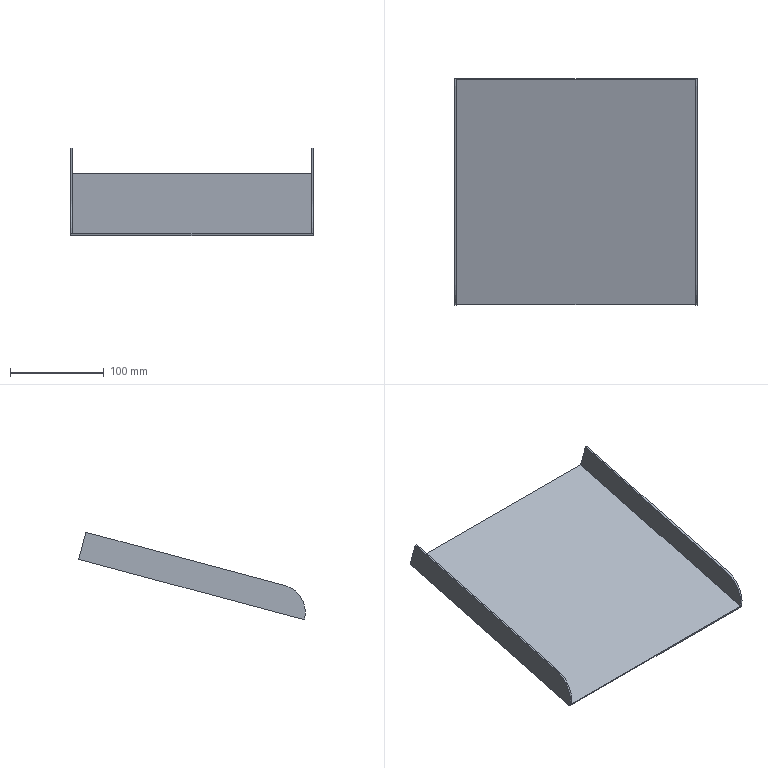Part | NX | features solid 2 | 1 solid | 12 faces | box 259.608 x 242.504 x 93.683 mm | volume 157032 mm3 | plane 10 | cylinder 2 | commonest cylinder face diameters 60 x2
STEP:
#1=CARTESIAN_POINT('',(828.,-707.325,-528.971));
#2=VERTEX_POINT('',#1);
#3=CARTESIAN_POINT('',(828.,-948.742,-593.658));
#4=VERTEX_POINT('',#3);
#5=CARTESIAN_POINT('',(828.,-784.599,-549.676));
#6=DIRECTION('',(0.,-0.9659,-0.2588));
#7=VECTOR('',#6,1000.);
#8=LINE('',#5,#7);
#9=EDGE_CURVE('',#2,#4,#8,.T.);
#10=ORIENTED_EDGE('',*,*,#9,.F.);
#11=CARTESIAN_POINT('',(572.392,-707.325,-528.971));
#12=VERTEX_POINT('',#11);
#13=CARTESIAN_POINT('',(818.,-707.325,-528.971));
#14=DIRECTION('',(1.,0.,0.));
#15=VECTOR('',#14,1000.);
#16=LINE('',#13,#15);
#17=EDGE_CURVE('',#2,#12,#16,.F.);
#18=ORIENTED_EDGE('',*,*,#17,.T.);
#19=CARTESIAN_POINT('',(572.392,-948.742,-593.658));
#20=VERTEX_POINT('',#19);
#21=CARTESIAN_POINT('',(572.392,-766.757,-544.895));
#22=DIRECTION('',(0.,0.9659,0.2588));
#23=VECTOR('',#22,1000.);
#24=LINE('',#21,#23);
#25=EDGE_CURVE('',#12,#20,#24,.F.);
#26=ORIENTED_EDGE('',*,*,#25,.T.);
#27=CARTESIAN_POINT('',(570.392,-948.742,-593.658));
#28=VERTEX_POINT('',#27);
#29=CARTESIAN_POINT('',(594.206,-948.742,-593.658));
#30=DIRECTION('',(-1.,0.,0.));
#31=VECTOR('',#30,1000.);
#32=LINE('',#29,#31);
#33=EDGE_CURVE('',#28,#20,#32,.F.);
#34=ORIENTED_EDGE('',*,*,#33,.F.);
#35=CARTESIAN_POINT('',(570.392,-948.807,-593.675));
#36=VERTEX_POINT('',#35);
#37=CARTESIAN_POINT('',(570.392,-795.624,-552.63));
#38=DIRECTION('',(0.,0.9659,0.2588));
#39=VECTOR('',#38,1000.);
#40=LINE('',#37,#39);
#41=EDGE_CURVE('',#28,#36,#40,.F.);
#42=ORIENTED_EDGE('',*,*,#41,.T.);
#43=CARTESIAN_POINT('',(830.,-948.807,-593.675));
#44=VERTEX_POINT('',#43);
#45=CARTESIAN_POINT('',(818.,-948.807,-593.675));
#46=DIRECTION('',(1.,0.,0.));
#47=VECTOR('',#46,1000.);
#48=LINE('',#45,#47);
#49=EDGE_CURVE('',#44,#36,#48,.F.);
#50=ORIENTED_EDGE('',*,*,#49,.F.);
#51=CARTESIAN_POINT('',(830.,-948.742,-593.658));
#52=VERTEX_POINT('',#51);
#53=CARTESIAN_POINT('',(830.,-784.599,-549.676));
#54=DIRECTION('',(0.,-0.9659,-0.2588));
#55=VECTOR('',#54,1000.);
#56=LINE('',#53,#55);
#57=EDGE_CURVE('',#52,#44,#56,.T.);
#58=ORIENTED_EDGE('',*,*,#57,.F.);
#59=CARTESIAN_POINT('',(830.,-948.742,-593.658));
#60=DIRECTION('',(1.,0.,0.));
#61=VECTOR('',#60,1000.);
#62=LINE('',#59,#61);
#63=EDGE_CURVE('',#4,#52,#62,.T.);
#64=ORIENTED_EDGE('',*,*,#63,.F.);
#65=EDGE_LOOP('',(#10,#18,#26,#34,#42,#50,#58,#64));
#66=FACE_BOUND('',#65,.T.);
#67=CARTESIAN_POINT('',(818.,-784.599,-549.676));
#68=DIRECTION('',(0.,-0.2588,0.9659));
#69=DIRECTION('',(1.,0.,0.));
#70=AXIS2_PLACEMENT_3D('',#67,#68,#69);
#71=PLANE('',#70);
#72=ADVANCED_FACE('',(#66),#71,.T.);
#73=ORIENTED_EDGE('',*,*,#17,.F.);
#74=CARTESIAN_POINT('',(828.,-714.572,-501.925));
#75=VERTEX_POINT('',#74);
#76=CARTESIAN_POINT('',(828.,-706.808,-530.902));
#77=DIRECTION('',(0.,0.2588,-0.9659));
#78=VECTOR('',#77,1000.);
#79=LINE('',#76,#78);
#80=EDGE_CURVE('',#2,#75,#79,.F.);
#81=ORIENTED_EDGE('',*,*,#80,.T.);
#82=CARTESIAN_POINT('',(830.,-714.572,-501.925));
#83=VERTEX_POINT('',#82);
#84=CARTESIAN_POINT('',(818.,-714.572,-501.925));
#85=DIRECTION('',(-1.,0.,0.));
#86=VECTOR('',#85,1000.);
#87=LINE('',#84,#86);
#88=EDGE_CURVE('',#83,#75,#87,.T.);
#89=ORIENTED_EDGE('',*,*,#88,.F.);
#90=CARTESIAN_POINT('',(830.,-706.808,-530.902));
#91=VERTEX_POINT('',#90);
#92=CARTESIAN_POINT('',(830.,-706.808,-530.902));
#93=DIRECTION('',(0.,0.2588,-0.9659));
#94=VECTOR('',#93,1000.);
#95=LINE('',#92,#94);
#96=EDGE_CURVE('',#91,#83,#95,.F.);
#97=ORIENTED_EDGE('',*,*,#96,.F.);
#98=CARTESIAN_POINT('',(570.392,-706.808,-530.902));
#99=VERTEX_POINT('',#98);
#100=CARTESIAN_POINT('',(818.,-706.808,-530.902));
#101=DIRECTION('',(1.,0.,0.));
#102=VECTOR('',#101,1000.);
#103=LINE('',#100,#102);
#104=EDGE_CURVE('',#91,#99,#103,.F.);
#105=ORIENTED_EDGE('',*,*,#104,.T.);
#106=CARTESIAN_POINT('',(570.392,-714.572,-501.925));
#107=VERTEX_POINT('',#106);
#108=CARTESIAN_POINT('',(570.392,-706.808,-530.902));
#109=DIRECTION('',(0.,-0.2588,0.9659));
#110=VECTOR('',#109,1000.);
#111=LINE('',#108,#110);
#112=EDGE_CURVE('',#99,#107,#111,.T.);
#113=ORIENTED_EDGE('',*,*,#112,.T.);
#114=CARTESIAN_POINT('',(572.392,-714.572,-501.925));
#115=VERTEX_POINT('',#114);
#116=CARTESIAN_POINT('',(818.,-714.572,-501.925));
#117=DIRECTION('',(-1.,0.,0.));
#118=VECTOR('',#117,1000.);
#119=LINE('',#116,#118);
#120=EDGE_CURVE('',#107,#115,#119,.F.);
#121=ORIENTED_EDGE('',*,*,#120,.T.);
#122=CARTESIAN_POINT('',(572.392,-706.808,-530.902));
#123=DIRECTION('',(0.,-0.2588,0.9659));
#124=VECTOR('',#123,1000.);
#125=LINE('',#122,#124);
#126=EDGE_CURVE('',#12,#115,#125,.T.);
#127=ORIENTED_EDGE('',*,*,#126,.F.);
#128=EDGE_LOOP('',(#73,#81,#89,#97,#105,#113,#121,#127));
#129=FACE_BOUND('',#128,.T.);
#130=CARTESIAN_POINT('',(818.,-706.808,-530.902));
#131=DIRECTION('',(0.,0.9659,0.2588));
#132=DIRECTION('',(-1.,0.,0.));
#133=AXIS2_PLACEMENT_3D('',#130,#131,#132);
#134=PLANE('',#133);
#135=ADVANCED_FACE('',(#129),#134,.T.);
#136=CARTESIAN_POINT('',(830.,-948.289,-595.607));
#137=VERTEX_POINT('',#136);
#138=CARTESIAN_POINT('',(830.,-948.289,-595.607));
#139=DIRECTION('',(0.,-0.2588,0.9659));
#140=VECTOR('',#139,1000.);
#141=LINE('',#138,#140);
#142=EDGE_CURVE('',#137,#44,#141,.T.);
#143=ORIENTED_EDGE('',*,*,#142,.F.);
#144=CARTESIAN_POINT('',(830.,-784.082,-551.608));
#145=DIRECTION('',(0.,-0.9659,-0.2588));
#146=VECTOR('',#145,1000.);
#147=LINE('',#144,#146);
#148=EDGE_CURVE('',#91,#137,#147,.T.);
#149=ORIENTED_EDGE('',*,*,#148,.F.);
#150=ORIENTED_EDGE('',*,*,#96,.T.);
#151=CARTESIAN_POINT('',(830.,-927.076,-558.865));
#152=VERTEX_POINT('',#151);
#153=CARTESIAN_POINT('',(830.,-791.846,-522.63));
#154=DIRECTION('',(0.,-0.9659,-0.2588));
#155=VECTOR('',#154,1000.);
#156=LINE('',#153,#155);
#157=EDGE_CURVE('',#83,#152,#156,.T.);
#158=ORIENTED_EDGE('',*,*,#157,.T.);
#159=CARTESIAN_POINT('',(830.,-919.311,-587.843));
#160=DIRECTION('',(-1.,0.,0.));
#161=DIRECTION('',(0.,-0.2588,0.9659));
#162=AXIS2_PLACEMENT_3D('',#159,#160,#161);
#163=CIRCLE('',#162,30.);
#164=EDGE_CURVE('',#152,#52,#163,.F.);
#165=ORIENTED_EDGE('',*,*,#164,.T.);
#166=ORIENTED_EDGE('',*,*,#57,.T.);
#167=EDGE_LOOP('',(#143,#149,#150,#158,#165,#166));
#168=FACE_BOUND('',#167,.T.);
#169=CARTESIAN_POINT('',(830.,-784.082,-551.608));
#170=DIRECTION('',(-1.,0.,0.));
#171=DIRECTION('',(0.,-0.9659,-0.2588));
#172=AXIS2_PLACEMENT_3D('',#169,#170,#171);
#173=PLANE('',#172);
#174=ADVANCED_FACE('',(#168),#173,.F.);
#175=ORIENTED_EDGE('',*,*,#142,.T.);
#176=ORIENTED_EDGE('',*,*,#49,.T.);
#177=CARTESIAN_POINT('',(570.392,-948.289,-595.607));
#178=VERTEX_POINT('',#177);
#179=CARTESIAN_POINT('',(570.392,-936.311,-640.312));
#180=DIRECTION('',(0.,0.2588,-0.9659));
#181=VECTOR('',#180,1000.);
#182=LINE('',#179,#181);
#183=EDGE_CURVE('',#178,#36,#182,.F.);
#184=ORIENTED_EDGE('',*,*,#183,.F.);
#185=CARTESIAN_POINT('',(818.,-948.289,-595.607));
#186=DIRECTION('',(-1.,0.,0.));
#187=VECTOR('',#186,1000.);
#188=LINE('',#185,#187);
#189=EDGE_CURVE('',#137,#178,#188,.T.);
#190=ORIENTED_EDGE('',*,*,#189,.F.);
#191=EDGE_LOOP('',(#175,#176,#184,#190));
#192=FACE_BOUND('',#191,.T.);
#193=CARTESIAN_POINT('',(818.,-948.289,-595.607));
#194=DIRECTION('',(0.,0.9659,0.2588));
#195=DIRECTION('',(-1.,0.,0.));
#196=AXIS2_PLACEMENT_3D('',#193,#194,#195);
#197=PLANE('',#196);
#198=ADVANCED_FACE('',(#192),#197,.F.);
#199=ORIENTED_EDGE('',*,*,#41,.F.);
#200=CARTESIAN_POINT('',(570.392,-927.076,-558.865));
#201=VERTEX_POINT('',#200);
#202=CARTESIAN_POINT('',(570.392,-919.311,-587.843));
#203=DIRECTION('',(-1.,0.,0.));
#204=DIRECTION('',(0.,0.,1.));
#205=AXIS2_PLACEMENT_3D('',#202,#203,#204);
#206=CIRCLE('',#205,30.);
#207=EDGE_CURVE('',#28,#201,#206,.T.);
#208=ORIENTED_EDGE('',*,*,#207,.T.);
#209=CARTESIAN_POINT('',(570.392,-791.846,-522.63));
#210=DIRECTION('',(0.,0.9659,0.2588));
#211=VECTOR('',#210,1000.);
#212=LINE('',#209,#211);
#213=EDGE_CURVE('',#107,#201,#212,.F.);
#214=ORIENTED_EDGE('',*,*,#213,.F.);
#215=ORIENTED_EDGE('',*,*,#112,.F.);
#216=CARTESIAN_POINT('',(570.392,-795.107,-554.562));
#217=DIRECTION('',(0.,0.9659,0.2588));
#218=VECTOR('',#217,1000.);
#219=LINE('',#216,#218);
#220=EDGE_CURVE('',#99,#178,#219,.F.);
#221=ORIENTED_EDGE('',*,*,#220,.T.);
#222=ORIENTED_EDGE('',*,*,#183,.T.);
#223=EDGE_LOOP('',(#199,#208,#214,#215,#221,#222));
#224=FACE_BOUND('',#223,.T.);
#225=CARTESIAN_POINT('',(570.392,-783.128,-599.267));
#226=DIRECTION('',(-1.,0.,0.));
#227=DIRECTION('',(0.,-0.9397,-0.342));
#228=AXIS2_PLACEMENT_3D('',#225,#226,#227);
#229=PLANE('',#228);
#230=ADVANCED_FACE('',(#224),#229,.T.);
#231=ORIENTED_EDGE('',*,*,#220,.F.);
#232=ORIENTED_EDGE('',*,*,#104,.F.);
#233=ORIENTED_EDGE('',*,*,#148,.T.);
#234=ORIENTED_EDGE('',*,*,#189,.T.);
#235=EDGE_LOOP('',(#231,#232,#233,#234));
#236=FACE_BOUND('',#235,.T.);
#237=CARTESIAN_POINT('',(818.,-784.082,-551.608));
#238=DIRECTION('',(0.,-0.2588,0.9659));
#239=DIRECTION('',(1.,0.,0.));
#240=AXIS2_PLACEMENT_3D('',#237,#238,#239);
#241=PLANE('',#240);
#242=ADVANCED_FACE('',(#236),#241,.F.);
#243=ORIENTED_EDGE('',*,*,#213,.T.);
#244=CARTESIAN_POINT('',(572.392,-927.076,-558.865));
#245=VERTEX_POINT('',#244);
#246=CARTESIAN_POINT('',(594.206,-927.076,-558.865));
#247=DIRECTION('',(-1.,0.,0.));
#248=VECTOR('',#247,1000.);
#249=LINE('',#246,#248);
#250=EDGE_CURVE('',#201,#245,#249,.F.);
#251=ORIENTED_EDGE('',*,*,#250,.T.);
#252=CARTESIAN_POINT('',(572.392,-791.846,-522.63));
#253=DIRECTION('',(0.,0.9659,0.2588));
#254=VECTOR('',#253,1000.);
#255=LINE('',#252,#254);
#256=EDGE_CURVE('',#115,#245,#255,.F.);
#257=ORIENTED_EDGE('',*,*,#256,.F.);
#258=ORIENTED_EDGE('',*,*,#120,.F.);
#259=EDGE_LOOP('',(#243,#251,#257,#258));
#260=FACE_BOUND('',#259,.T.);
#261=CARTESIAN_POINT('',(594.206,-791.846,-522.63));
#262=DIRECTION('',(0.,0.2588,-0.9659));
#263=DIRECTION('',(0.,-0.9659,-0.2588));
#264=AXIS2_PLACEMENT_3D('',#261,#262,#263);
#265=PLANE('',#264);
#266=ADVANCED_FACE('',(#260),#265,.F.);
#267=ORIENTED_EDGE('',*,*,#25,.F.);
#268=ORIENTED_EDGE('',*,*,#126,.T.);
#269=ORIENTED_EDGE('',*,*,#256,.T.);
#270=CARTESIAN_POINT('',(572.392,-919.311,-587.843));
#271=DIRECTION('',(-1.,0.,0.));
#272=DIRECTION('',(0.,0.,1.));
#273=AXIS2_PLACEMENT_3D('',#270,#271,#272);
#274=CIRCLE('',#273,30.);
#275=EDGE_CURVE('',#245,#20,#274,.F.);
#276=ORIENTED_EDGE('',*,*,#275,.T.);
#277=EDGE_LOOP('',(#267,#268,#269,#276));
#278=FACE_BOUND('',#277,.T.);
#279=CARTESIAN_POINT('',(572.392,-754.937,-589.006));
#280=DIRECTION('',(-1.,0.,0.));
#281=DIRECTION('',(0.,0.,1.));
#282=AXIS2_PLACEMENT_3D('',#279,#280,#281);
#283=PLANE('',#282);
#284=ADVANCED_FACE('',(#278),#283,.F.);
#285=ORIENTED_EDGE('',*,*,#207,.F.);
#286=ORIENTED_EDGE('',*,*,#33,.T.);
#287=ORIENTED_EDGE('',*,*,#275,.F.);
#288=ORIENTED_EDGE('',*,*,#250,.F.);
#289=EDGE_LOOP('',(#285,#286,#287,#288));
#290=FACE_BOUND('',#289,.T.);
#291=CARTESIAN_POINT('',(594.206,-919.311,-587.843));
#292=DIRECTION('',(-1.,0.,0.));
#293=DIRECTION('',(0.,-0.2588,0.9659));
#294=AXIS2_PLACEMENT_3D('',#291,#292,#293);
#295=CYLINDRICAL_SURFACE('',#294,30.);
#296=ADVANCED_FACE('',(#290),#295,.T.);
#297=CARTESIAN_POINT('',(828.,-927.076,-558.865));
#298=VERTEX_POINT('',#297);
#299=CARTESIAN_POINT('',(828.,-791.846,-522.63));
#300=DIRECTION('',(0.,0.9659,0.2588));
#301=VECTOR('',#300,1000.);
#302=LINE('',#299,#301);
#303=EDGE_CURVE('',#75,#298,#302,.F.);
#304=ORIENTED_EDGE('',*,*,#303,.T.);
#305=CARTESIAN_POINT('',(830.,-927.076,-558.865));
#306=DIRECTION('',(-1.,0.,0.));
#307=VECTOR('',#306,1000.);
#308=LINE('',#305,#307);
#309=EDGE_CURVE('',#298,#152,#308,.F.);
#310=ORIENTED_EDGE('',*,*,#309,.T.);
#311=ORIENTED_EDGE('',*,*,#157,.F.);
#312=ORIENTED_EDGE('',*,*,#88,.T.);
#313=EDGE_LOOP('',(#304,#310,#311,#312));
#314=FACE_BOUND('',#313,.T.);
#315=CARTESIAN_POINT('',(830.,-791.846,-522.63));
#316=DIRECTION('',(0.,0.2588,-0.9659));
#317=DIRECTION('',(0.,-0.9659,-0.2588));
#318=AXIS2_PLACEMENT_3D('',#315,#316,#317);
#319=PLANE('',#318);
#320=ADVANCED_FACE('',(#314),#319,.F.);
#321=ORIENTED_EDGE('',*,*,#80,.F.);
#322=ORIENTED_EDGE('',*,*,#9,.T.);
#323=CARTESIAN_POINT('',(828.,-919.311,-587.843));
#324=DIRECTION('',(-1.,0.,0.));
#325=DIRECTION('',(0.,-0.2588,0.9659));
#326=AXIS2_PLACEMENT_3D('',#323,#324,#325);
#327=CIRCLE('',#326,30.);
#328=EDGE_CURVE('',#4,#298,#327,.T.);
#329=ORIENTED_EDGE('',*,*,#328,.T.);
#330=ORIENTED_EDGE('',*,*,#303,.F.);
#331=EDGE_LOOP('',(#321,#322,#329,#330));
#332=FACE_BOUND('',#331,.T.);
#333=CARTESIAN_POINT('',(828.,-784.082,-551.608));
#334=DIRECTION('',(-1.,0.,0.));
#335=DIRECTION('',(0.,-0.2588,0.9659));
#336=AXIS2_PLACEMENT_3D('',#333,#334,#335);
#337=PLANE('',#336);
#338=ADVANCED_FACE('',(#332),#337,.T.);
#339=ORIENTED_EDGE('',*,*,#328,.F.);
#340=ORIENTED_EDGE('',*,*,#63,.T.);
#341=ORIENTED_EDGE('',*,*,#164,.F.);
#342=ORIENTED_EDGE('',*,*,#309,.F.);
#343=EDGE_LOOP('',(#339,#340,#341,#342));
#344=FACE_BOUND('',#343,.T.);
#345=CARTESIAN_POINT('',(830.,-919.311,-587.843));
#346=DIRECTION('',(1.,0.,0.));
#347=DIRECTION('',(0.,0.2588,-0.9659));
#348=AXIS2_PLACEMENT_3D('',#345,#346,#347);
#349=CYLINDRICAL_SURFACE('',#348,30.);
#350=ADVANCED_FACE('',(#344),#349,.T.);
#351=CLOSED_SHELL('',(#72,#135,#174,#198,#230,#242,#266,#284,#296,#320,#338,#350));
#352=MANIFOLD_SOLID_BREP('',#351);
#353=(LENGTH_UNIT()NAMED_UNIT(*)SI_UNIT(.MILLI.,.METRE.));
#354=UNCERTAINTY_MEASURE_WITH_UNIT(LENGTH_MEASURE(0.00001),#353,'','');
#355=(NAMED_UNIT(*)PLANE_ANGLE_UNIT()SI_UNIT($,.RADIAN.));
#356=(NAMED_UNIT(*)SI_UNIT($,.STERADIAN.)SOLID_ANGLE_UNIT());
#357=(GEOMETRIC_REPRESENTATION_CONTEXT(3)GLOBAL_UNCERTAINTY_ASSIGNED_CONTEXT((#354))GLOBAL_UNIT_ASSIGNED_CONTEXT((#353,#355,#356))REPRESENTATION_CONTEXT('',''));
#358=ADVANCED_BREP_SHAPE_REPRESENTATION('',(#352),#357);